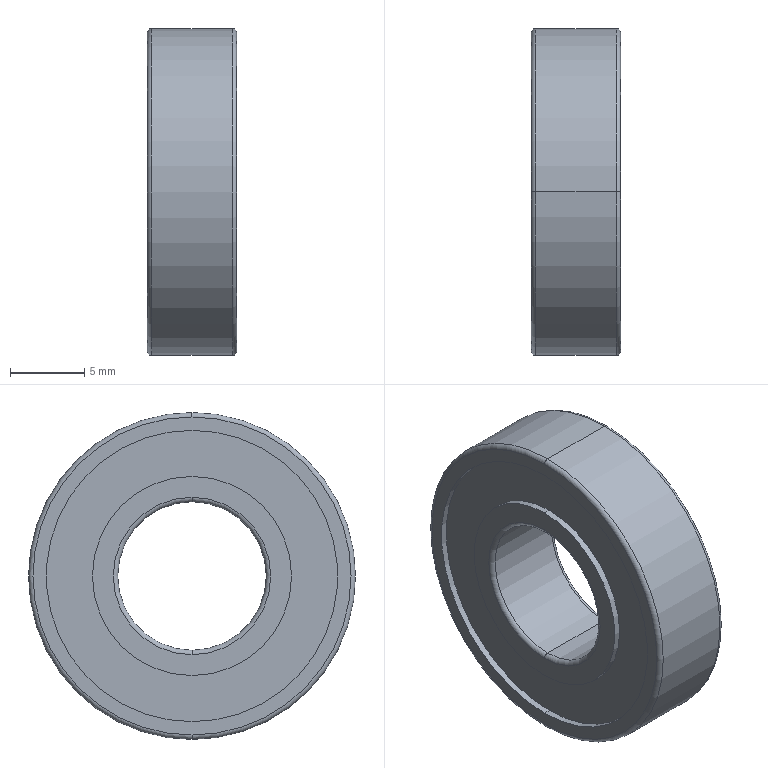Part | STEP file | Bearing seat bearing_6900 V1.201001 | 1 solid | 26 faces | box 6 x 22 x 22 mm | volume 1661 mm3 | cylinder 12 | torus 8 | plane 6 | commonest cylinder face diameters 13.4 x4 19.6 x4 10 x2 22 x2